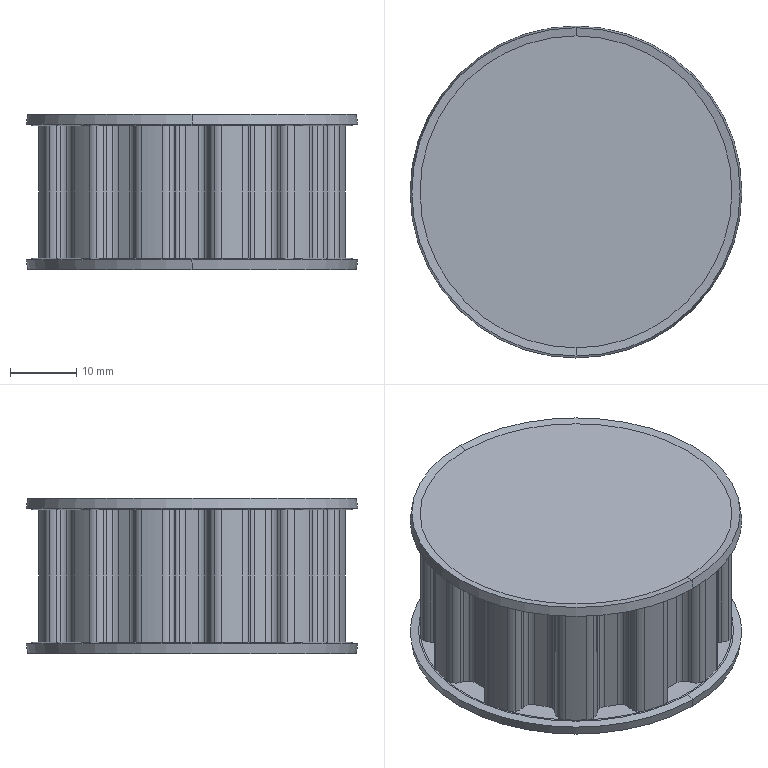Part | SolidWorks | features BaseBody 1 | 1 solid | 186 faces | box 50.139 x 50.139 x 23.437 mm | volume 36944 mm3 | cylinder 108 | plane 62 | cone 12 | torus 4 | commonest cylinder face diameters 3.2 x96 47.139 x12